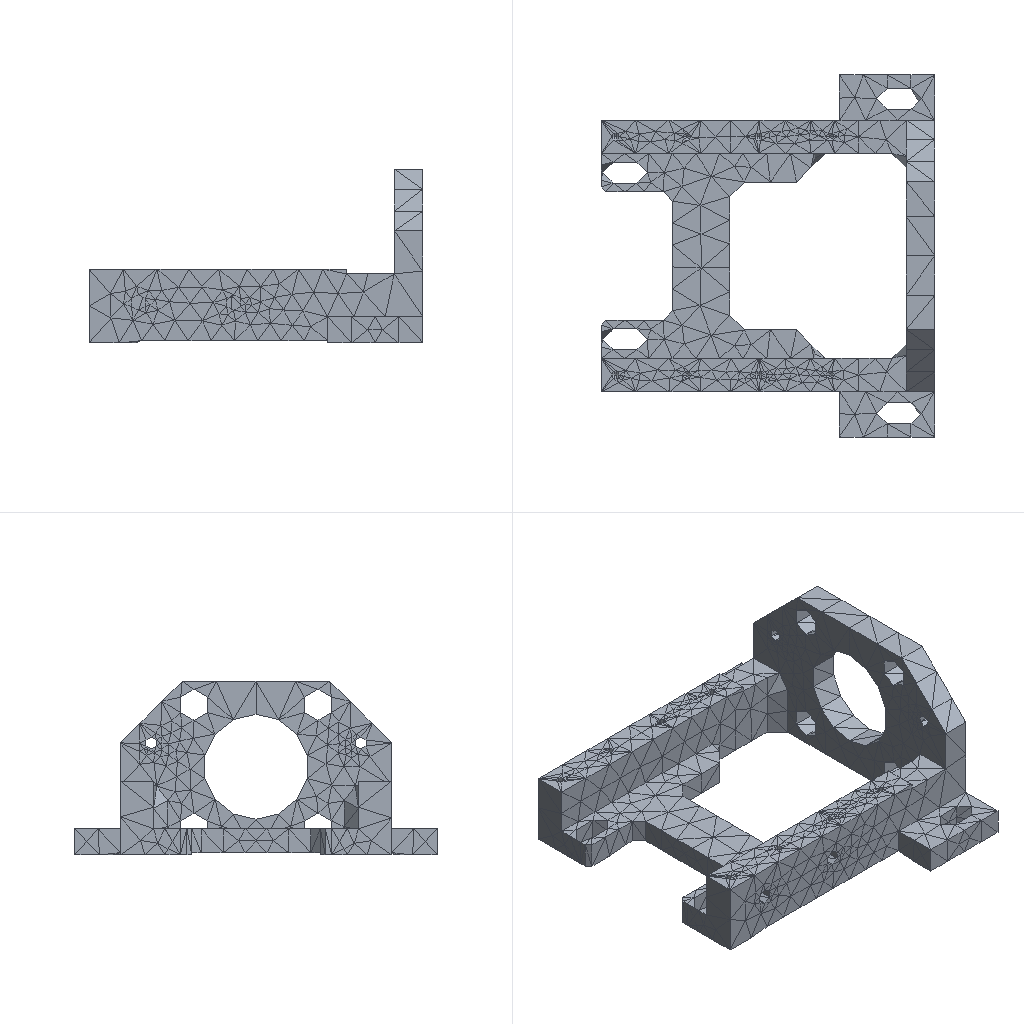Simulation study | nx simcenter
Set-up summary:
category,name,step,type,value,unit,region
solver,nx_nastran (Simcenter)
units,not stated in the deck,,not stated
analysis,deck,,static,static
analysis,solution,,SOL,101
load_step,SUBCASE 1,1,SUBCASE,SPC=1 LOAD=2
load_step,requested,,,1
mesh,nodes,,,6591
mesh,elements,,,3267
element_type,CTETRA,,solid,3267
load,nodal force total,,FX,0.0,model units
load,nodal force total,,FY,0.0,model units
load,nodal force total,,FZ,2000000.057,model units
load,load commands in deck,,count,271
bc,support commands in deck,,count,632
analysis,NX solution 0,,Structural,Linear Statics - Single Constraint
check,setup vs results,,match,every grid point's frame and coordinates and every element id; grid points of CTETRA elements
Nastran input file, long lists of numbers shortened:
$*$$$$$$$$$$$$$$$$$$$$$$$$$$$$$$$$$$$$$$$$$$$$$$$$$$$$$$$$$$$$$$$$$
$*
$*                    NX v10.0.0.24 TRANSLATOR
$*                    FOR NX NASTRAN VERSION 10.0
$ (33 more lines like these left out)
ASSIGN OUTPUT2='123_sim1-solution_1.op2' UNIT=12
$*
$*$$$$$$$$$$$$$$$$$$$$$$$$$$$$$$$$$$$
$*
$* EXECUTIVE CONTROL
$*
$*$$$$$$$$$$$$$$$$$$$$$$$$$$$$$$$$$$$
$*
ID,NASTRAN,123_sim1-solution_1
SOL 101
CEND
$*
$*$$$$$$$$$$$$$$$$$$$$$$$$$$$$$$$$$$$
$*
$* CASE CONTROL
$*
$*$$$$$$$$$$$$$$$$$$$$$$$$$$$$$$$$$$$
$*
TITLE = Solution 1
ECHO = NONE
SPC = 1
OUTPUT
BCRESULTS(TRACTION,FORCE,PLOT) = ALL
DISPLACEMENT(PLOT) = ALL
ESE(PLOT) = ALL
FORCE(PLOT,CORNER) = ALL
OLOAD(PLOT) = ALL
SPCFORCES(PLOT) = ALL
STRAIN(PLOT,FIBER,CORNER) = ALL
STRESS(PLOT,CORNER) = ALL
$*  NX Step: Subcase - Static Loads 1
SUBCASE 1
LABEL = Subcase - Static Loads 1
LOAD = 2
$*
$*$$$$$$$$$$$$$$$$$$$$$$$$$$$$$$$$$$$
$*
$* BULK DATA
$*
$*$$$$$$$$$$$$$$$$$$$$$$$$$$$$$$$$$$$
$*
BEGIN BULK
$*
$* PARAM CARDS
$*
PARAM      K6ROT100.0000
PARAM     OIBULK     YES
PARAM    OMACHPR     YES
PARAM       POST      -2
PARAM    POSTEXT     YES
PARAM    UNITSYS   MN-MM
$*
$* GRID CARDS
$*
GRID*               6424               00.0000000000E+001.2500000000E+01+
*       1.5000000000E+01               0
GRID*               6425               02.8421709430E-141.2500000000E+01+
*       -5.000000000E-01               0
$ (13178 more lines like these left out)
$*
$* ELEMENT CARDS
$*
$*  NX Mesh Collector: Solid(1)
$*  NX Mesh: 3d_mesh(1)
CTETRA         1       1    2778       1    2777       2     118     119+
+           2885     120     121     122
CTETRA         2       1    5355    6448       3    5359     123     124+
+            125    2456     126     127
$ (6530 more lines like these left out)
$*
$* PROPERTY CARDS
$*
$*  NX Property: PSOLID1
PSOLID         1       1       0                           SMECH
$*
$* MATERIAL CARDS
$*
$*  NX Material: Aluminum_6061
MAT1           16.8980+7        0.3300002.7110-62.2161-5
MATT1          1       1               2               3
TABLEM1        1                                                        +
+        20.00006.8980+7 21.11006.8980+7 23.89006.8980+7 37.78006.8290+7+
+        51.67006.8290+7 65.56006.7600+7 79.44006.6910+7 93.33006.6221+7+
+       107.22006.5531+7121.11006.4841+7135.00006.4151+7148.89006.3461+7+
+       162.78006.2772+7176.67006.1392+7190.56006.0702+7204.44005.9323+7+
+       218.33005.8633+7232.22005.7253+7246.11005.5874+7260.00005.4494+7+
+       273.89005.3114+7287.78005.1735+7301.67005.0355+7315.56004.8976+7+
+       329.44004.7596+7343.33004.6216+7357.22004.4147+7371.11004.2767+7+
+       385.00004.1388+7398.89003.9318+7412.78003.7939+7426.67003.5869+7+
+           ENDT
TABLEM1        2                                                        +
+        20.00000.330000 21.11000.330000    ENDT
TABLEM1        3                                                        +
+        20.00002.2380-5 93.33002.3184-5107.22002.3346-5121.11002.3508-5+
+       135.00002.3670-5148.89002.3832-5162.78002.3994-5176.67002.4138-5+
+       190.56002.4300-5204.44002.4444-5218.33002.4588-5232.22002.4732-5+
+       246.11002.4876-5260.00002.5002-5273.89002.5146-5287.78002.5272-5+
+       301.67002.5398-5315.56002.5524-5    ENDT
$*
$* LOAD AND CONSTRAINT CARDS
$*
$*  NX Load and Constraint: Fixed(1)
SPC            1    4907  123456  0.0000
SPC            1    4908  123456  0.0000
SPC            1    4909  123456  0.0000
SPC            1    4910  123456  0.0000
$ (628 more lines like these left out)
$*  NX Load and Constraint: Force(1)
FORCE          2    3267       015711.78  0.0000  0.00001.000000
FORCE          2    3268       012138.90  0.0000  0.00001.000000
FORCE          2    3269       015502.10  0.0000  0.00001.000000
FORCE          2    3270       019750.44  0.0000  0.00001.000000
$ (267 more lines like these left out)
ENDDATA 766c5125
Results summary:
result,analysis,,,static
result,last_loadstep,,,1
result,primary field,,,displacements
result,max displacement,,,0.3123,model units
result,reaction total,,FX,0.3297,model units
result,reaction total,,FY,-0.03909,model units
result,reaction total,,FZ,-2000000.125,model units
result,NX solution 0,,loadcases,1,mm